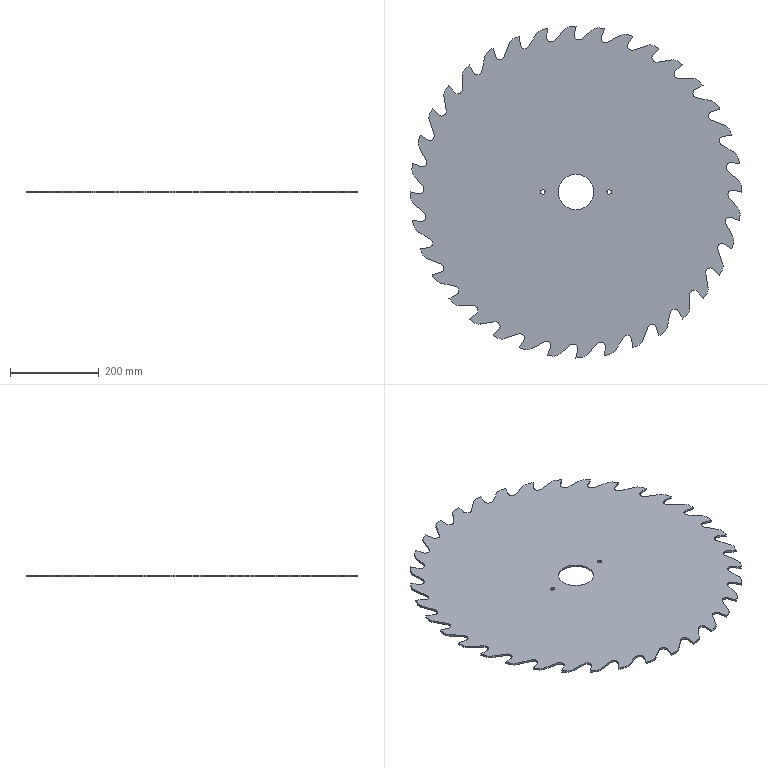Part | SolidWorks | features Cut 1, Extrusion 1 | 1 solid | 206 faces | box 750 x 750 x 4 mm | volume 1607952 mm3 | plane 110 | cylinder 96 | commonest cylinder face diameters 20 x50 40 x40 10 x4 80 x2